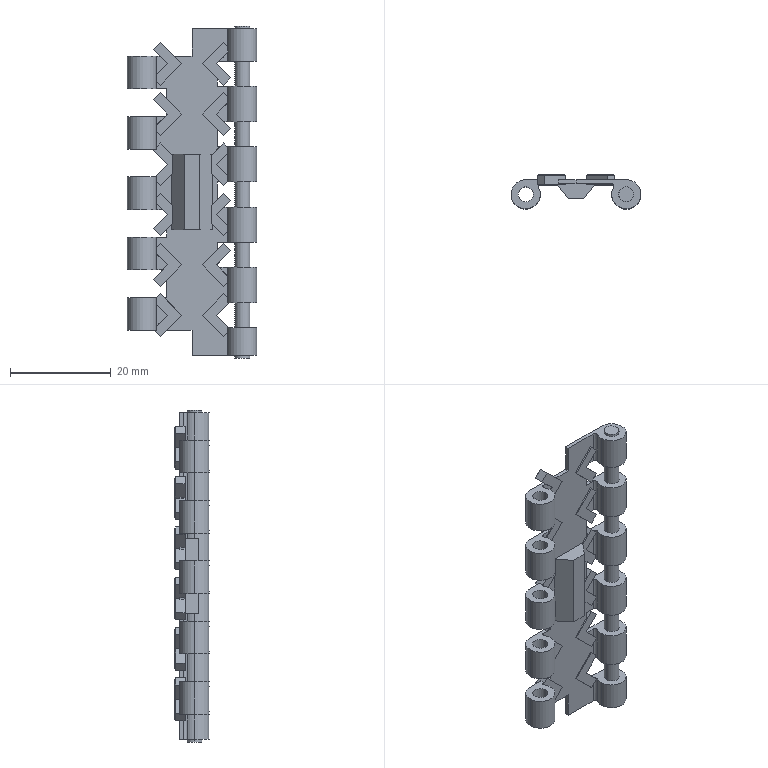Part | SolidWorks | features ICE 7, Chamfer 1, Extrusion 1 | 2 solids | 354 faces | box 25.8 x 6.8 x 66 mm | volume 3099 mm3 | plane 281 | cylinder 73 | commonest cylinder face diameters 5.8 x33 3 x22 1.032 x16 2.95 x2